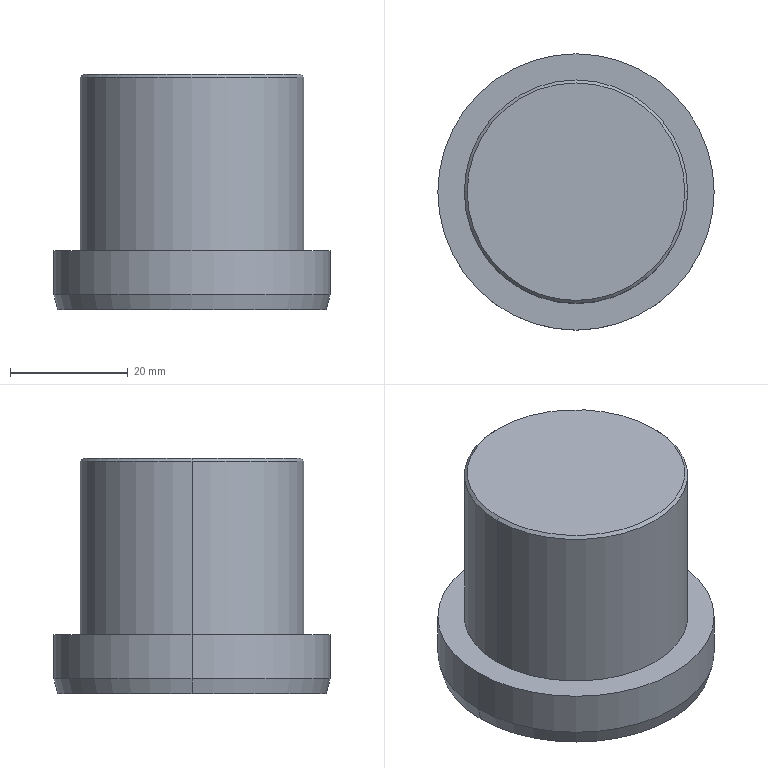Part | NX | features MYKP38-200_3 2 | 1 solid | 11 faces | box 47 x 47 x 40 mm | volume 51236 mm3 | cylinder 4 | cone 4 | plane 3 | commonest cylinder face diameters 38 x2 47 x2
STEP:
#1=CARTESIAN_POINT('',(1778.977,-312.405,-180.001));
#2=VERTEX_POINT('',#1);
#3=CARTESIAN_POINT('',(1778.977,-312.405,-150.501));
#4=VERTEX_POINT('',#3);
#5=CARTESIAN_POINT('',(1778.977,-312.405,-180.001));
#6=DIRECTION('',(0.00000006,0.,1.));
#7=VECTOR('',#6,1000.);
#8=LINE('',#5,#7);
#9=EDGE_CURVE('',#2,#4,#8,.T.);
#10=ORIENTED_EDGE('',*,*,#9,.T.);
#11=CARTESIAN_POINT('',(1740.977,-312.405,-150.501));
#12=VERTEX_POINT('',#11);
#13=CARTESIAN_POINT('',(1759.977,-312.405,-150.501));
#14=DIRECTION('',(0.,0.,-1.));
#15=DIRECTION('',(1.,0.,0.));
#16=AXIS2_PLACEMENT_3D('',#13,#14,#15);
#17=CIRCLE('',#16,19.);
#18=EDGE_CURVE('',#4,#12,#17,.T.);
#19=ORIENTED_EDGE('',*,*,#18,.T.);
#20=CARTESIAN_POINT('',(1740.977,-312.405,-180.001));
#21=VERTEX_POINT('',#20);
#22=CARTESIAN_POINT('',(1740.977,-312.405,-180.001));
#23=DIRECTION('',(-0.00000006,0.,1.));
#24=VECTOR('',#23,1000.);
#25=LINE('',#22,#24);
#26=EDGE_CURVE('',#12,#21,#25,.F.);
#27=ORIENTED_EDGE('',*,*,#26,.T.);
#28=CARTESIAN_POINT('',(1759.977,-312.405,-180.001));
#29=DIRECTION('',(0.,0.,1.));
#30=DIRECTION('',(-1.,0.,0.));
#31=AXIS2_PLACEMENT_3D('',#28,#29,#30);
#32=CIRCLE('',#31,19.);
#33=EDGE_CURVE('',#21,#2,#32,.T.);
#34=ORIENTED_EDGE('',*,*,#33,.T.);
#35=EDGE_LOOP('',(#10,#19,#27,#34));
#36=FACE_BOUND('',#35,.T.);
#37=CARTESIAN_POINT('',(1759.977,-312.405,-150.001));
#38=DIRECTION('',(0.,0.,1.));
#39=DIRECTION('',(1.,0.,0.));
#40=AXIS2_PLACEMENT_3D('',#37,#38,#39);
#41=CYLINDRICAL_SURFACE('',#40,19.);
#42=ADVANCED_FACE('',(#36),#41,.T.);
#43=CARTESIAN_POINT('',(1778.477,-312.405,-150.001));
#44=VERTEX_POINT('',#43);
#45=CARTESIAN_POINT('',(1778.477,-312.405,-150.001));
#46=DIRECTION('',(0.7071,-0.000000002,-0.7071));
#47=VECTOR('',#46,1000.);
#48=LINE('',#45,#47);
#49=EDGE_CURVE('',#44,#4,#48,.T.);
#50=ORIENTED_EDGE('',*,*,#49,.F.);
#51=CARTESIAN_POINT('',(1741.477,-312.405,-150.001));
#52=VERTEX_POINT('',#51);
#53=CARTESIAN_POINT('',(1759.977,-312.405,-150.001));
#54=DIRECTION('',(0.,0.,-1.));
#55=DIRECTION('',(1.,0.,0.));
#56=AXIS2_PLACEMENT_3D('',#53,#54,#55);
#57=CIRCLE('',#56,18.5);
#58=EDGE_CURVE('',#44,#52,#57,.T.);
#59=ORIENTED_EDGE('',*,*,#58,.T.);
#60=CARTESIAN_POINT('',(1741.477,-312.405,-150.001));
#61=DIRECTION('',(-0.7071,0.000000002,-0.7071));
#62=VECTOR('',#61,1000.);
#63=LINE('',#60,#62);
#64=EDGE_CURVE('',#12,#52,#63,.F.);
#65=ORIENTED_EDGE('',*,*,#64,.F.);
#66=ORIENTED_EDGE('',*,*,#18,.F.);
#67=EDGE_LOOP('',(#50,#59,#65,#66));
#68=FACE_BOUND('',#67,.T.);
#69=CARTESIAN_POINT('',(1759.977,-312.405,-150.251));
#70=DIRECTION('',(0.,0.,-1.));
#71=DIRECTION('',(0.,-1.,0.));
#72=AXIS2_PLACEMENT_3D('',#69,#70,#71);
#73=CONICAL_SURFACE('',#72,18.75,0.7854);
#74=ADVANCED_FACE('',(#68),#73,.T.);
#75=ORIENTED_EDGE('',*,*,#58,.F.);
#76=CARTESIAN_POINT('',(1759.977,-312.405,-150.001));
#77=DIRECTION('',(0.,0.,-1.));
#78=DIRECTION('',(-1.,0.,0.));
#79=AXIS2_PLACEMENT_3D('',#76,#77,#78);
#80=CIRCLE('',#79,18.5);
#81=EDGE_CURVE('',#52,#44,#80,.T.);
#82=ORIENTED_EDGE('',*,*,#81,.F.);
#83=EDGE_LOOP('',(#75,#82));
#84=FACE_BOUND('',#83,.T.);
#85=CARTESIAN_POINT('',(1759.977,-312.405,-150.001));
#86=DIRECTION('',(0.,0.,1.));
#87=DIRECTION('',(0.,-1.,0.));
#88=AXIS2_PLACEMENT_3D('',#85,#86,#87);
#89=PLANE('',#88);
#90=ADVANCED_FACE('',(#84),#89,.T.);
#91=ORIENTED_EDGE('',*,*,#64,.T.);
#92=ORIENTED_EDGE('',*,*,#81,.T.);
#93=ORIENTED_EDGE('',*,*,#49,.T.);
#94=CARTESIAN_POINT('',(1759.977,-312.405,-150.501));
#95=DIRECTION('',(0.,0.,-1.));
#96=DIRECTION('',(-1.,0.,0.));
#97=AXIS2_PLACEMENT_3D('',#94,#95,#96);
#98=CIRCLE('',#97,19.);
#99=EDGE_CURVE('',#12,#4,#98,.T.);
#100=ORIENTED_EDGE('',*,*,#99,.F.);
#101=EDGE_LOOP('',(#91,#92,#93,#100));
#102=FACE_BOUND('',#101,.T.);
#103=CARTESIAN_POINT('',(1759.977,-312.405,-150.251));
#104=DIRECTION('',(0.,0.,-1.));
#105=DIRECTION('',(0.,-1.,0.));
#106=AXIS2_PLACEMENT_3D('',#103,#104,#105);
#107=CONICAL_SURFACE('',#106,18.75,0.7854);
#108=ADVANCED_FACE('',(#102),#107,.T.);
#109=ORIENTED_EDGE('',*,*,#26,.F.);
#110=ORIENTED_EDGE('',*,*,#99,.T.);
#111=ORIENTED_EDGE('',*,*,#9,.F.);
#112=CARTESIAN_POINT('',(1759.977,-312.405,-180.001));
#113=DIRECTION('',(0.,0.,1.));
#114=DIRECTION('',(1.,0.,0.));
#115=AXIS2_PLACEMENT_3D('',#112,#113,#114);
#116=CIRCLE('',#115,19.);
#117=EDGE_CURVE('',#2,#21,#116,.T.);
#118=ORIENTED_EDGE('',*,*,#117,.T.);
#119=EDGE_LOOP('',(#109,#110,#111,#118));
#120=FACE_BOUND('',#119,.T.);
#121=CARTESIAN_POINT('',(1759.977,-312.405,-150.001));
#122=DIRECTION('',(0.,0.,1.));
#123=DIRECTION('',(1.,0.,0.));
#124=AXIS2_PLACEMENT_3D('',#121,#122,#123);
#125=CYLINDRICAL_SURFACE('',#124,19.);
#126=ADVANCED_FACE('',(#120),#125,.T.);
#127=CARTESIAN_POINT('',(1736.477,-312.405,-180.001));
#128=VERTEX_POINT('',#127);
#129=CARTESIAN_POINT('',(1783.477,-312.405,-180.001));
#130=VERTEX_POINT('',#129);
#131=CARTESIAN_POINT('',(1759.977,-312.405,-180.001));
#132=DIRECTION('',(0.,0.,-1.));
#133=DIRECTION('',(-1.,0.,0.));
#134=AXIS2_PLACEMENT_3D('',#131,#132,#133);
#135=CIRCLE('',#134,23.5);
#136=EDGE_CURVE('',#128,#130,#135,.T.);
#137=ORIENTED_EDGE('',*,*,#136,.F.);
#138=CARTESIAN_POINT('',(1759.977,-312.405,-180.001));
#139=DIRECTION('',(0.,0.,-1.));
#140=DIRECTION('',(1.,0.,0.));
#141=AXIS2_PLACEMENT_3D('',#138,#139,#140);
#142=CIRCLE('',#141,23.5);
#143=EDGE_CURVE('',#130,#128,#142,.T.);
#144=ORIENTED_EDGE('',*,*,#143,.F.);
#145=EDGE_LOOP('',(#137,#144));
#146=FACE_BOUND('',#145,.T.);
#147=ORIENTED_EDGE('',*,*,#33,.F.);
#148=ORIENTED_EDGE('',*,*,#117,.F.);
#149=EDGE_LOOP('',(#147,#148));
#150=FACE_BOUND('',#149,.T.);
#151=CARTESIAN_POINT('',(1759.977,-312.405,-180.001));
#152=DIRECTION('',(0.,0.,1.));
#153=DIRECTION('',(0.,-1.,0.));
#154=AXIS2_PLACEMENT_3D('',#151,#152,#153);
#155=PLANE('',#154);
#156=ADVANCED_FACE('',(#146,#150),#155,.T.);
#157=CARTESIAN_POINT('',(1736.477,-312.405,-187.501));
#158=VERTEX_POINT('',#157);
#159=CARTESIAN_POINT('',(1783.477,-312.405,-187.501));
#160=VERTEX_POINT('',#159);
#161=CARTESIAN_POINT('',(1759.977,-312.405,-187.501));
#162=DIRECTION('',(0.,0.,1.));
#163=DIRECTION('',(-1.,0.,0.));
#164=AXIS2_PLACEMENT_3D('',#161,#162,#163);
#165=CIRCLE('',#164,23.5);
#166=EDGE_CURVE('',#158,#160,#165,.T.);
#167=ORIENTED_EDGE('',*,*,#166,.T.);
#168=CARTESIAN_POINT('',(1783.477,-312.405,-187.501));
#169=DIRECTION('',(0.,0.,1.));
#170=VECTOR('',#169,1000.);
#171=LINE('',#168,#170);
#172=EDGE_CURVE('',#130,#160,#171,.F.);
#173=ORIENTED_EDGE('',*,*,#172,.F.);
#174=ORIENTED_EDGE('',*,*,#143,.T.);
#175=CARTESIAN_POINT('',(1736.477,-312.405,-187.501));
#176=DIRECTION('',(0.,0.,1.));
#177=VECTOR('',#176,1000.);
#178=LINE('',#175,#177);
#179=EDGE_CURVE('',#158,#128,#178,.T.);
#180=ORIENTED_EDGE('',*,*,#179,.F.);
#181=EDGE_LOOP('',(#167,#173,#174,#180));
#182=FACE_BOUND('',#181,.T.);
#183=CARTESIAN_POINT('',(1759.977,-312.405,-180.001));
#184=DIRECTION('',(0.,0.,1.));
#185=DIRECTION('',(1.,0.,0.));
#186=AXIS2_PLACEMENT_3D('',#183,#184,#185);
#187=CYLINDRICAL_SURFACE('',#186,23.5);
#188=ADVANCED_FACE('',(#182),#187,.T.);
#189=ORIENTED_EDGE('',*,*,#136,.T.);
#190=ORIENTED_EDGE('',*,*,#172,.T.);
#191=CARTESIAN_POINT('',(1759.977,-312.405,-187.501));
#192=DIRECTION('',(0.,0.,1.));
#193=DIRECTION('',(1.,0.,0.));
#194=AXIS2_PLACEMENT_3D('',#191,#192,#193);
#195=CIRCLE('',#194,23.5);
#196=EDGE_CURVE('',#160,#158,#195,.T.);
#197=ORIENTED_EDGE('',*,*,#196,.T.);
#198=ORIENTED_EDGE('',*,*,#179,.T.);
#199=EDGE_LOOP('',(#189,#190,#197,#198));
#200=FACE_BOUND('',#199,.T.);
#201=CARTESIAN_POINT('',(1759.977,-312.405,-180.001));
#202=DIRECTION('',(0.,0.,1.));
#203=DIRECTION('',(1.,0.,0.));
#204=AXIS2_PLACEMENT_3D('',#201,#202,#203);
#205=CYLINDRICAL_SURFACE('',#204,23.5);
#206=ADVANCED_FACE('',(#200),#205,.T.);
#207=ORIENTED_EDGE('',*,*,#196,.F.);
#208=CARTESIAN_POINT('',(1782.807,-312.405,-190.001));
#209=VERTEX_POINT('',#208);
#210=CARTESIAN_POINT('',(1782.807,-312.405,-190.001));
#211=DIRECTION('',(0.2588,0.,0.9659));
#212=VECTOR('',#211,1000.);
#213=LINE('',#210,#212);
#214=EDGE_CURVE('',#160,#209,#213,.F.);
#215=ORIENTED_EDGE('',*,*,#214,.T.);
#216=CARTESIAN_POINT('',(1737.147,-312.405,-190.001));
#217=VERTEX_POINT('',#216);
#218=CARTESIAN_POINT('',(1759.977,-312.405,-190.001));
#219=DIRECTION('',(0.,0.,1.));
#220=DIRECTION('',(1.,0.,0.));
#221=AXIS2_PLACEMENT_3D('',#218,#219,#220);
#222=CIRCLE('',#221,22.83);
#223=EDGE_CURVE('',#209,#217,#222,.T.);
#224=ORIENTED_EDGE('',*,*,#223,.T.);
#225=CARTESIAN_POINT('',(1737.147,-312.405,-190.001));
#226=DIRECTION('',(-0.2588,0.,0.9659));
#227=VECTOR('',#226,1000.);
#228=LINE('',#225,#227);
#229=EDGE_CURVE('',#217,#158,#228,.T.);
#230=ORIENTED_EDGE('',*,*,#229,.T.);
#231=EDGE_LOOP('',(#207,#215,#224,#230));
#232=FACE_BOUND('',#231,.T.);
#233=CARTESIAN_POINT('',(1759.977,-312.405,-188.751));
#234=DIRECTION('',(0.,0.,1.));
#235=DIRECTION('',(-1.,0.,0.));
#236=AXIS2_PLACEMENT_3D('',#233,#234,#235);
#237=CONICAL_SURFACE('',#236,23.165,0.2618);
#238=ADVANCED_FACE('',(#232),#237,.T.);
#239=CARTESIAN_POINT('',(1759.977,-335.235,-190.001));
#240=VERTEX_POINT('',#239);
#241=CARTESIAN_POINT('',(1759.977,-312.405,-190.001));
#242=DIRECTION('',(0.,0.,1.));
#243=DIRECTION('',(0.,-1.,0.));
#244=AXIS2_PLACEMENT_3D('',#241,#242,#243);
#245=CIRCLE('',#244,22.83);
#246=EDGE_CURVE('',#240,#209,#245,.T.);
#247=ORIENTED_EDGE('',*,*,#246,.T.);
#248=ORIENTED_EDGE('',*,*,#214,.F.);
#249=ORIENTED_EDGE('',*,*,#166,.F.);
#250=ORIENTED_EDGE('',*,*,#229,.F.);
#251=CARTESIAN_POINT('',(1759.977,-312.405,-190.001));
#252=DIRECTION('',(0.,0.,1.));
#253=DIRECTION('',(-1.,0.,0.));
#254=AXIS2_PLACEMENT_3D('',#251,#252,#253);
#255=CIRCLE('',#254,22.83);
#256=EDGE_CURVE('',#217,#240,#255,.T.);
#257=ORIENTED_EDGE('',*,*,#256,.T.);
#258=EDGE_LOOP('',(#247,#248,#249,#250,#257));
#259=FACE_BOUND('',#258,.T.);
#260=CARTESIAN_POINT('',(1759.977,-312.405,-188.751));
#261=DIRECTION('',(0.,0.,1.));
#262=DIRECTION('',(-1.,0.,0.));
#263=AXIS2_PLACEMENT_3D('',#260,#261,#262);
#264=CONICAL_SURFACE('',#263,23.165,0.2618);
#265=ADVANCED_FACE('',(#259),#264,.T.);
#266=ORIENTED_EDGE('',*,*,#246,.F.);
#267=ORIENTED_EDGE('',*,*,#256,.F.);
#268=ORIENTED_EDGE('',*,*,#223,.F.);
#269=EDGE_LOOP('',(#266,#267,#268));
#270=FACE_BOUND('',#269,.T.);
#271=CARTESIAN_POINT('',(1759.977,-312.405,-190.001));
#272=DIRECTION('',(0.,0.,-1.));
#273=DIRECTION('',(1.,0.,0.));
#274=AXIS2_PLACEMENT_3D('',#271,#272,#273);
#275=PLANE('',#274);
#276=ADVANCED_FACE('',(#270),#275,.T.);
#277=CLOSED_SHELL('',(#42,#74,#90,#108,#126,#156,#188,#206,#238,#265,#276));
#278=MANIFOLD_SOLID_BREP('',#277);
#279=(LENGTH_UNIT()NAMED_UNIT(*)SI_UNIT(.MILLI.,.METRE.));
#280=UNCERTAINTY_MEASURE_WITH_UNIT(LENGTH_MEASURE(0.00001),#279,'','');
#281=(NAMED_UNIT(*)PLANE_ANGLE_UNIT()SI_UNIT($,.RADIAN.));
#282=(NAMED_UNIT(*)SI_UNIT($,.STERADIAN.)SOLID_ANGLE_UNIT());
#283=(GEOMETRIC_REPRESENTATION_CONTEXT(3)GLOBAL_UNCERTAINTY_ASSIGNED_CONTEXT((#280))GLOBAL_UNIT_ASSIGNED_CONTEXT((#279,#281,#282))REPRESENTATION_CONTEXT('',''));
#284=ADVANCED_BREP_SHAPE_REPRESENTATION('',(#278),#283);